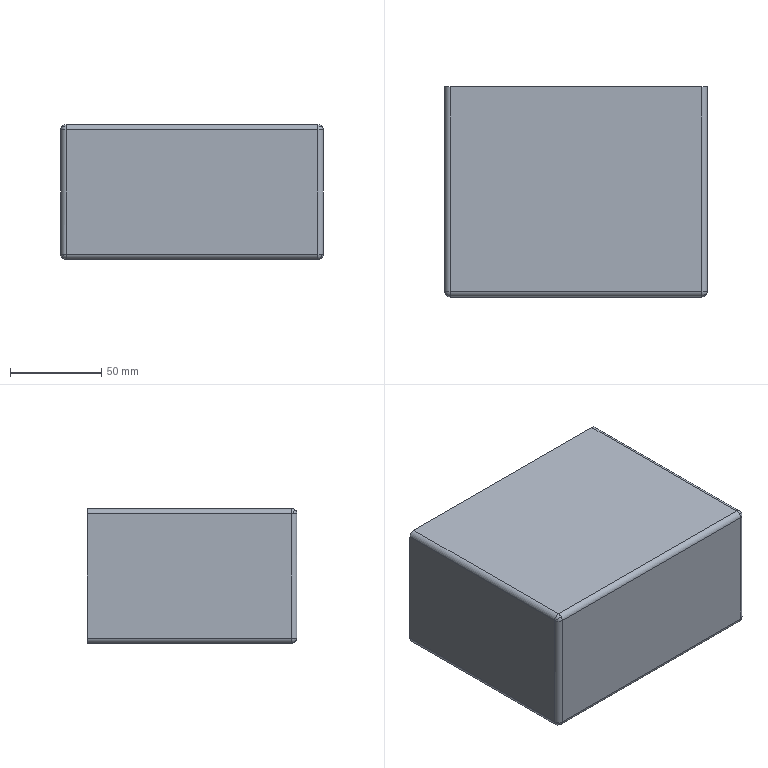Part | SolidWorks | features BaseBody 1 | 1 solid | 22 faces | box 144 x 115 x 74 mm | volume 1223728 mm3 | sphere 8 | cylinder 8 | plane 6 | commonest cylinder face diameters 6 x8
STEP:
#1=CARTESIAN_POINT('',(69.,-150.,-34.));
#2=VERTEX_POINT('',#1);
#3=CARTESIAN_POINT('',(69.,-147.,-37.));
#4=VERTEX_POINT('',#3);
#5=CARTESIAN_POINT('',(69.,-147.,-34.));
#6=DIRECTION('',(1.,0.,0.));
#7=DIRECTION('',(0.,-1.,0.));
#8=AXIS2_PLACEMENT_3D('',#5,#6,#7);
#9=CIRCLE('',#8,3.);
#10=EDGE_CURVE('',#2,#4,#9,.T.);
#11=ORIENTED_EDGE('',*,*,#10,.T.);
#12=CARTESIAN_POINT('',(71.121,-149.121,-34.));
#13=VERTEX_POINT('',#12);
#14=CARTESIAN_POINT('',(69.,-147.,-34.));
#15=DIRECTION('',(-0.7071,-0.7071,0.));
#16=DIRECTION('',(0.7071,-0.7071,0.));
#17=AXIS2_PLACEMENT_3D('',#14,#15,#16);
#18=CIRCLE('',#17,3.);
#19=EDGE_CURVE('',#4,#13,#18,.T.);
#20=ORIENTED_EDGE('',*,*,#19,.T.);
#21=CARTESIAN_POINT('',(69.,-147.,-34.));
#22=DIRECTION('',(0.,0.,-1.));
#23=DIRECTION('',(1.,0.,0.));
#24=AXIS2_PLACEMENT_3D('',#21,#22,#23);
#25=CIRCLE('',#24,3.);
#26=EDGE_CURVE('',#13,#2,#25,.T.);
#27=ORIENTED_EDGE('',*,*,#26,.T.);
#28=EDGE_LOOP('',(#11,#20,#27));
#29=FACE_OUTER_BOUND('',#28,.T.);
#30=CARTESIAN_POINT('',(69.,-147.,-34.));
#31=DIRECTION('',(-0.7071,-0.7071,0.));
#32=DIRECTION('',(-0.5774,0.5774,0.5774));
#33=AXIS2_PLACEMENT_3D('',#30,#31,#32);
#34=SPHERICAL_SURFACE('',#33,3.);
#35=ADVANCED_FACE('',(#29),#34,.T.);
#36=CARTESIAN_POINT('',(69.,-147.,37.));
#37=VERTEX_POINT('',#36);
#38=CARTESIAN_POINT('',(69.,-149.121,36.121));
#39=VERTEX_POINT('',#38);
#40=CARTESIAN_POINT('',(69.,-147.,34.));
#41=DIRECTION('',(1.,0.,0.));
#42=DIRECTION('',(0.,0.,1.));
#43=AXIS2_PLACEMENT_3D('',#40,#41,#42);
#44=CIRCLE('',#43,3.);
#45=EDGE_CURVE('',#37,#39,#44,.T.);
#46=ORIENTED_EDGE('',*,*,#45,.T.);
#47=CARTESIAN_POINT('',(72.,-147.,34.));
#48=VERTEX_POINT('',#47);
#49=CARTESIAN_POINT('',(69.,-147.,34.));
#50=DIRECTION('',(0.,0.7071,0.7071));
#51=DIRECTION('',(0.,-0.7071,0.7071));
#52=AXIS2_PLACEMENT_3D('',#49,#50,#51);
#53=CIRCLE('',#52,3.);
#54=EDGE_CURVE('',#39,#48,#53,.T.);
#55=ORIENTED_EDGE('',*,*,#54,.T.);
#56=CARTESIAN_POINT('',(69.,-147.,34.));
#57=DIRECTION('',(0.,-1.,0.));
#58=DIRECTION('',(1.,0.,0.));
#59=AXIS2_PLACEMENT_3D('',#56,#57,#58);
#60=CIRCLE('',#59,3.);
#61=EDGE_CURVE('',#48,#37,#60,.T.);
#62=ORIENTED_EDGE('',*,*,#61,.T.);
#63=EDGE_LOOP('',(#46,#55,#62));
#64=FACE_OUTER_BOUND('',#63,.T.);
#65=CARTESIAN_POINT('',(69.,-147.,34.));
#66=DIRECTION('',(0.,0.7071,0.7071));
#67=DIRECTION('',(-0.5774,0.5774,-0.5774));
#68=AXIS2_PLACEMENT_3D('',#65,#66,#67);
#69=SPHERICAL_SURFACE('',#68,3.);
#70=ADVANCED_FACE('',(#64),#69,.T.);
#71=CARTESIAN_POINT('',(-69.,-150.,-34.));
#72=VERTEX_POINT('',#71);
#73=CARTESIAN_POINT('',(-70.342,-149.683,-34.));
#74=VERTEX_POINT('',#73);
#75=CARTESIAN_POINT('',(-69.,-147.,-34.));
#76=DIRECTION('',(0.,0.,-1.));
#77=DIRECTION('',(0.,-1.,0.));
#78=AXIS2_PLACEMENT_3D('',#75,#76,#77);
#79=CIRCLE('',#78,3.);
#80=EDGE_CURVE('',#72,#74,#79,.T.);
#81=ORIENTED_EDGE('',*,*,#80,.T.);
#82=CARTESIAN_POINT('',(-70.342,-147.,-36.683));
#83=VERTEX_POINT('',#82);
#84=CARTESIAN_POINT('',(-69.,-147.,-34.));
#85=DIRECTION('',(0.8165,-0.4082,-0.4082));
#86=DIRECTION('',(0.4472,0.8944,0.));
#87=AXIS2_PLACEMENT_3D('',#84,#85,#86);
#88=CIRCLE('',#87,3.);
#89=EDGE_CURVE('',#74,#83,#88,.T.);
#90=ORIENTED_EDGE('',*,*,#89,.T.);
#91=CARTESIAN_POINT('',(-69.,-147.,-37.));
#92=VERTEX_POINT('',#91);
#93=CARTESIAN_POINT('',(-69.,-147.,-34.));
#94=DIRECTION('',(0.,-1.,0.));
#95=DIRECTION('',(-1.,0.,0.));
#96=AXIS2_PLACEMENT_3D('',#93,#94,#95);
#97=CIRCLE('',#96,3.);
#98=EDGE_CURVE('',#83,#92,#97,.T.);
#99=ORIENTED_EDGE('',*,*,#98,.T.);
#100=CARTESIAN_POINT('',(-69.,-147.,-34.));
#101=DIRECTION('',(-1.,0.,0.));
#102=DIRECTION('',(0.,0.,-1.));
#103=AXIS2_PLACEMENT_3D('',#100,#101,#102);
#104=CIRCLE('',#103,3.);
#105=EDGE_CURVE('',#92,#72,#104,.T.);
#106=ORIENTED_EDGE('',*,*,#105,.T.);
#107=EDGE_LOOP('',(#81,#90,#99,#106));
#108=FACE_OUTER_BOUND('',#107,.T.);
#109=CARTESIAN_POINT('',(-69.,-147.,-34.));
#110=DIRECTION('',(0.8165,-0.4082,-0.4082));
#111=DIRECTION('',(0.5774,0.5774,0.5774));
#112=AXIS2_PLACEMENT_3D('',#109,#110,#111);
#113=SPHERICAL_SURFACE('',#112,3.);
#114=ADVANCED_FACE('',(#108),#113,.T.);
#115=CARTESIAN_POINT('',(-69.,-147.,37.));
#116=VERTEX_POINT('',#115);
#117=CARTESIAN_POINT('',(-72.,-147.,34.));
#118=VERTEX_POINT('',#117);
#119=CARTESIAN_POINT('',(-69.,-147.,34.));
#120=DIRECTION('',(0.,-1.,0.));
#121=DIRECTION('',(0.,0.,1.));
#122=AXIS2_PLACEMENT_3D('',#119,#120,#121);
#123=CIRCLE('',#122,3.);
#124=EDGE_CURVE('',#116,#118,#123,.T.);
#125=ORIENTED_EDGE('',*,*,#124,.T.);
#126=CARTESIAN_POINT('',(-69.,-149.121,36.121));
#127=VERTEX_POINT('',#126);
#128=CARTESIAN_POINT('',(-69.,-147.,34.));
#129=DIRECTION('',(0.,0.7071,0.7071));
#130=DIRECTION('',(0.,-0.7071,0.7071));
#131=AXIS2_PLACEMENT_3D('',#128,#129,#130);
#132=CIRCLE('',#131,3.);
#133=EDGE_CURVE('',#118,#127,#132,.T.);
#134=ORIENTED_EDGE('',*,*,#133,.T.);
#135=CARTESIAN_POINT('',(-69.,-147.,34.));
#136=DIRECTION('',(-1.,0.,0.));
#137=DIRECTION('',(0.,-1.,0.));
#138=AXIS2_PLACEMENT_3D('',#135,#136,#137);
#139=CIRCLE('',#138,3.);
#140=EDGE_CURVE('',#127,#116,#139,.T.);
#141=ORIENTED_EDGE('',*,*,#140,.T.);
#142=EDGE_LOOP('',(#125,#134,#141));
#143=FACE_OUTER_BOUND('',#142,.T.);
#144=CARTESIAN_POINT('',(-69.,-147.,34.));
#145=DIRECTION('',(0.,0.7071,0.7071));
#146=DIRECTION('',(0.5774,0.5774,-0.5774));
#147=AXIS2_PLACEMENT_3D('',#144,#145,#146);
#148=SPHERICAL_SURFACE('',#147,3.);
#149=ADVANCED_FACE('',(#143),#148,.T.);
#150=CARTESIAN_POINT('',(-72.,-35.,34.));
#151=VERTEX_POINT('',#150);
#152=CARTESIAN_POINT('',(-72.,-35.,34.));
#153=DIRECTION('',(0.,-1.,0.));
#154=VECTOR('',#153,1000.);
#155=LINE('',#152,#154);
#156=EDGE_CURVE('',#151,#118,#155,.T.);
#157=ORIENTED_EDGE('',*,*,#156,.F.);
#158=CARTESIAN_POINT('',(-72.,-35.,-34.));
#159=VERTEX_POINT('',#158);
#160=CARTESIAN_POINT('',(-72.,-35.,-34.));
#161=DIRECTION('',(0.,0.,1.));
#162=VECTOR('',#161,1000.);
#163=LINE('',#160,#162);
#164=EDGE_CURVE('',#159,#151,#163,.T.);
#165=ORIENTED_EDGE('',*,*,#164,.F.);
#166=CARTESIAN_POINT('',(-72.,-147.,-34.));
#167=VERTEX_POINT('',#166);
#168=CARTESIAN_POINT('',(-72.,-147.,-34.));
#169=DIRECTION('',(0.,1.,0.));
#170=VECTOR('',#169,1000.);
#171=LINE('',#168,#170);
#172=EDGE_CURVE('',#167,#159,#171,.T.);
#173=ORIENTED_EDGE('',*,*,#172,.F.);
#174=CARTESIAN_POINT('',(-72.,-147.,34.));
#175=DIRECTION('',(0.,0.,-1.));
#176=VECTOR('',#175,1000.);
#177=LINE('',#174,#176);
#178=EDGE_CURVE('',#118,#167,#177,.T.);
#179=ORIENTED_EDGE('',*,*,#178,.F.);
#180=EDGE_LOOP('',(#157,#165,#173,#179));
#181=FACE_OUTER_BOUND('',#180,.T.);
#182=CARTESIAN_POINT('',(-72.,-150.,-37.));
#183=DIRECTION('',(-1.,0.,0.));
#184=DIRECTION('',(0.,0.,1.));
#185=AXIS2_PLACEMENT_3D('',#182,#183,#184);
#186=PLANE('',#185);
#187=ADVANCED_FACE('',(#181),#186,.T.);
#188=CARTESIAN_POINT('',(69.,-35.,37.));
#189=VERTEX_POINT('',#188);
#190=CARTESIAN_POINT('',(69.,-35.,37.));
#191=DIRECTION('',(0.,-1.,0.));
#192=VECTOR('',#191,1000.);
#193=LINE('',#190,#192);
#194=EDGE_CURVE('',#189,#37,#193,.T.);
#195=ORIENTED_EDGE('',*,*,#194,.F.);
#196=CARTESIAN_POINT('',(-69.,-35.,37.));
#197=VERTEX_POINT('',#196);
#198=CARTESIAN_POINT('',(-69.,-35.,37.));
#199=DIRECTION('',(1.,0.,0.));
#200=VECTOR('',#199,1000.);
#201=LINE('',#198,#200);
#202=EDGE_CURVE('',#197,#189,#201,.T.);
#203=ORIENTED_EDGE('',*,*,#202,.F.);
#204=CARTESIAN_POINT('',(-69.,-147.,37.));
#205=DIRECTION('',(0.,1.,0.));
#206=VECTOR('',#205,1000.);
#207=LINE('',#204,#206);
#208=EDGE_CURVE('',#116,#197,#207,.T.);
#209=ORIENTED_EDGE('',*,*,#208,.F.);
#210=CARTESIAN_POINT('',(69.,-147.,37.));
#211=DIRECTION('',(-1.,0.,0.));
#212=VECTOR('',#211,1000.);
#213=LINE('',#210,#212);
#214=EDGE_CURVE('',#37,#116,#213,.T.);
#215=ORIENTED_EDGE('',*,*,#214,.F.);
#216=EDGE_LOOP('',(#195,#203,#209,#215));
#217=FACE_OUTER_BOUND('',#216,.T.);
#218=CARTESIAN_POINT('',(-72.,-150.,37.));
#219=DIRECTION('',(0.,0.,1.));
#220=DIRECTION('',(1.,0.,0.));
#221=AXIS2_PLACEMENT_3D('',#218,#219,#220);
#222=PLANE('',#221);
#223=ADVANCED_FACE('',(#217),#222,.T.);
#224=CARTESIAN_POINT('',(-69.,-150.,34.));
#225=VERTEX_POINT('',#224);
#226=CARTESIAN_POINT('',(-69.,-150.,-34.));
#227=DIRECTION('',(0.,0.,1.));
#228=VECTOR('',#227,1000.);
#229=LINE('',#226,#228);
#230=EDGE_CURVE('',#72,#225,#229,.T.);
#231=ORIENTED_EDGE('',*,*,#230,.F.);
#232=CARTESIAN_POINT('',(69.,-150.,-34.));
#233=DIRECTION('',(-1.,0.,0.));
#234=VECTOR('',#233,1000.);
#235=LINE('',#232,#234);
#236=EDGE_CURVE('',#2,#72,#235,.T.);
#237=ORIENTED_EDGE('',*,*,#236,.F.);
#238=CARTESIAN_POINT('',(69.,-150.,34.));
#239=VERTEX_POINT('',#238);
#240=CARTESIAN_POINT('',(69.,-150.,34.));
#241=DIRECTION('',(0.,0.,-1.));
#242=VECTOR('',#241,1000.);
#243=LINE('',#240,#242);
#244=EDGE_CURVE('',#239,#2,#243,.T.);
#245=ORIENTED_EDGE('',*,*,#244,.F.);
#246=CARTESIAN_POINT('',(-69.,-150.,34.));
#247=DIRECTION('',(1.,0.,0.));
#248=VECTOR('',#247,1000.);
#249=LINE('',#246,#248);
#250=EDGE_CURVE('',#225,#239,#249,.T.);
#251=ORIENTED_EDGE('',*,*,#250,.F.);
#252=EDGE_LOOP('',(#231,#237,#245,#251));
#253=FACE_OUTER_BOUND('',#252,.T.);
#254=CARTESIAN_POINT('',(0.,-150.,0.));
#255=DIRECTION('',(0.,-1.,0.));
#256=DIRECTION('',(0.,0.,-1.));
#257=AXIS2_PLACEMENT_3D('',#254,#255,#256);
#258=PLANE('',#257);
#259=ADVANCED_FACE('',(#253),#258,.T.);
#260=CARTESIAN_POINT('',(72.,-35.,34.));
#261=VERTEX_POINT('',#260);
#262=CARTESIAN_POINT('',(69.,-35.,34.));
#263=DIRECTION('',(0.,-1.,0.));
#264=DIRECTION('',(1.,0.,0.));
#265=AXIS2_PLACEMENT_3D('',#262,#263,#264);
#266=CIRCLE('',#265,3.);
#267=EDGE_CURVE('',#261,#189,#266,.T.);
#268=ORIENTED_EDGE('',*,*,#267,.F.);
#269=CARTESIAN_POINT('',(72.,-35.,-34.));
#270=VERTEX_POINT('',#269);
#271=CARTESIAN_POINT('',(72.,-35.,-34.));
#272=DIRECTION('',(0.,0.,1.));
#273=VECTOR('',#272,1000.);
#274=LINE('',#271,#273);
#275=EDGE_CURVE('',#270,#261,#274,.T.);
#276=ORIENTED_EDGE('',*,*,#275,.F.);
#277=CARTESIAN_POINT('',(69.,-35.,-37.));
#278=VERTEX_POINT('',#277);
#279=CARTESIAN_POINT('',(69.,-35.,-34.));
#280=DIRECTION('',(0.,-1.,0.));
#281=DIRECTION('',(0.,0.,-1.));
#282=AXIS2_PLACEMENT_3D('',#279,#280,#281);
#283=CIRCLE('',#282,3.);
#284=EDGE_CURVE('',#278,#270,#283,.T.);
#285=ORIENTED_EDGE('',*,*,#284,.F.);
#286=CARTESIAN_POINT('',(-69.,-35.,-37.));
#287=VERTEX_POINT('',#286);
#288=CARTESIAN_POINT('',(-69.,-35.,-37.));
#289=DIRECTION('',(1.,0.,0.));
#290=VECTOR('',#289,1000.);
#291=LINE('',#288,#290);
#292=EDGE_CURVE('',#287,#278,#291,.T.);
#293=ORIENTED_EDGE('',*,*,#292,.F.);
#294=CARTESIAN_POINT('',(-69.,-35.,-34.));
#295=DIRECTION('',(0.,-1.,0.));
#296=DIRECTION('',(-1.,0.,0.));
#297=AXIS2_PLACEMENT_3D('',#294,#295,#296);
#298=CIRCLE('',#297,3.);
#299=EDGE_CURVE('',#159,#287,#298,.T.);
#300=ORIENTED_EDGE('',*,*,#299,.F.);
#301=ORIENTED_EDGE('',*,*,#164,.T.);
#302=CARTESIAN_POINT('',(-69.,-35.,34.));
#303=DIRECTION('',(0.,-1.,0.));
#304=DIRECTION('',(0.,0.,1.));
#305=AXIS2_PLACEMENT_3D('',#302,#303,#304);
#306=CIRCLE('',#305,3.);
#307=EDGE_CURVE('',#197,#151,#306,.T.);
#308=ORIENTED_EDGE('',*,*,#307,.F.);
#309=ORIENTED_EDGE('',*,*,#202,.T.);
#310=EDGE_LOOP('',(#268,#276,#285,#293,#300,#301,#308,#309));
#311=FACE_OUTER_BOUND('',#310,.T.);
#312=CARTESIAN_POINT('',(0.,-35.,0.));
#313=DIRECTION('',(0.,1.,0.));
#314=DIRECTION('',(1.,0.,0.));
#315=AXIS2_PLACEMENT_3D('',#312,#313,#314);
#316=PLANE('',#315);
#317=ADVANCED_FACE('',(#311),#316,.T.);
#318=CARTESIAN_POINT('',(69.,-147.,-37.));
#319=DIRECTION('',(0.,1.,0.));
#320=VECTOR('',#319,1000.);
#321=LINE('',#318,#320);
#322=EDGE_CURVE('',#4,#278,#321,.T.);
#323=ORIENTED_EDGE('',*,*,#322,.F.);
#324=CARTESIAN_POINT('',(-69.,-147.,-37.));
#325=DIRECTION('',(1.,0.,0.));
#326=VECTOR('',#325,1000.);
#327=LINE('',#324,#326);
#328=EDGE_CURVE('',#92,#4,#327,.T.);
#329=ORIENTED_EDGE('',*,*,#328,.F.);
#330=CARTESIAN_POINT('',(-69.,-35.,-37.));
#331=DIRECTION('',(0.,-1.,0.));
#332=VECTOR('',#331,1000.);
#333=LINE('',#330,#332);
#334=EDGE_CURVE('',#287,#92,#333,.T.);
#335=ORIENTED_EDGE('',*,*,#334,.F.);
#336=ORIENTED_EDGE('',*,*,#292,.T.);
#337=EDGE_LOOP('',(#323,#329,#335,#336));
#338=FACE_OUTER_BOUND('',#337,.T.);
#339=CARTESIAN_POINT('',(72.,-150.,-37.));
#340=DIRECTION('',(0.,0.,-1.));
#341=DIRECTION('',(0.,-1.,0.));
#342=AXIS2_PLACEMENT_3D('',#339,#340,#341);
#343=PLANE('',#342);
#344=ADVANCED_FACE('',(#338),#343,.T.);
#345=CARTESIAN_POINT('',(72.,-147.,34.));
#346=DIRECTION('',(0.,1.,0.));
#347=VECTOR('',#346,1000.);
#348=LINE('',#345,#347);
#349=EDGE_CURVE('',#48,#261,#348,.T.);
#350=ORIENTED_EDGE('',*,*,#349,.F.);
#351=CARTESIAN_POINT('',(72.,-147.,-34.));
#352=VERTEX_POINT('',#351);
#353=CARTESIAN_POINT('',(72.,-147.,-34.));
#354=DIRECTION('',(0.,0.,1.));
#355=VECTOR('',#354,1000.);
#356=LINE('',#353,#355);
#357=EDGE_CURVE('',#352,#48,#356,.T.);
#358=ORIENTED_EDGE('',*,*,#357,.F.);
#359=CARTESIAN_POINT('',(72.,-35.,-34.));
#360=DIRECTION('',(0.,-1.,0.));
#361=VECTOR('',#360,1000.);
#362=LINE('',#359,#361);
#363=EDGE_CURVE('',#270,#352,#362,.T.);
#364=ORIENTED_EDGE('',*,*,#363,.F.);
#365=ORIENTED_EDGE('',*,*,#275,.T.);
#366=EDGE_LOOP('',(#350,#358,#364,#365));
#367=FACE_OUTER_BOUND('',#366,.T.);
#368=CARTESIAN_POINT('',(72.,-150.,37.));
#369=DIRECTION('',(1.,0.,0.));
#370=DIRECTION('',(0.,0.,1.));
#371=AXIS2_PLACEMENT_3D('',#368,#369,#370);
#372=PLANE('',#371);
#373=ADVANCED_FACE('',(#367),#372,.T.);
#374=ORIENTED_EDGE('',*,*,#284,.T.);
#375=ORIENTED_EDGE('',*,*,#363,.T.);
#376=CARTESIAN_POINT('',(69.,-147.,-34.));
#377=DIRECTION('',(0.,-1.,0.));
#378=DIRECTION('',(0.,0.,-1.));
#379=AXIS2_PLACEMENT_3D('',#376,#377,#378);
#380=CIRCLE('',#379,3.);
#381=EDGE_CURVE('',#4,#352,#380,.T.);
#382=ORIENTED_EDGE('',*,*,#381,.F.);
#383=ORIENTED_EDGE('',*,*,#322,.T.);
#384=EDGE_LOOP('',(#374,#375,#382,#383));
#385=FACE_OUTER_BOUND('',#384,.T.);
#386=CARTESIAN_POINT('',(69.,-147.,-34.));
#387=DIRECTION('',(0.,1.,0.));
#388=DIRECTION('',(0.,0.,-1.));
#389=AXIS2_PLACEMENT_3D('',#386,#387,#388);
#390=CYLINDRICAL_SURFACE('',#389,3.);
#391=ADVANCED_FACE('',(#385),#390,.T.);
#392=ORIENTED_EDGE('',*,*,#105,.F.);
#393=ORIENTED_EDGE('',*,*,#328,.T.);
#394=ORIENTED_EDGE('',*,*,#10,.F.);
#395=ORIENTED_EDGE('',*,*,#236,.T.);
#396=EDGE_LOOP('',(#392,#393,#394,#395));
#397=FACE_OUTER_BOUND('',#396,.T.);
#398=CARTESIAN_POINT('',(69.,-147.,-34.));
#399=DIRECTION('',(-1.,0.,0.));
#400=DIRECTION('',(0.,-1.,0.));
#401=AXIS2_PLACEMENT_3D('',#398,#399,#400);
#402=CYLINDRICAL_SURFACE('',#401,3.);
#403=ADVANCED_FACE('',(#397),#402,.T.);
#404=ORIENTED_EDGE('',*,*,#299,.T.);
#405=ORIENTED_EDGE('',*,*,#334,.T.);
#406=ORIENTED_EDGE('',*,*,#98,.F.);
#407=CARTESIAN_POINT('',(-69.,-147.,-34.));
#408=DIRECTION('',(0.,-1.,0.));
#409=DIRECTION('',(-1.,0.,0.));
#410=AXIS2_PLACEMENT_3D('',#407,#408,#409);
#411=CIRCLE('',#410,3.);
#412=EDGE_CURVE('',#167,#83,#411,.T.);
#413=ORIENTED_EDGE('',*,*,#412,.F.);
#414=ORIENTED_EDGE('',*,*,#172,.T.);
#415=EDGE_LOOP('',(#404,#405,#406,#413,#414));
#416=FACE_OUTER_BOUND('',#415,.T.);
#417=CARTESIAN_POINT('',(-69.,-147.,-34.));
#418=DIRECTION('',(0.,1.,0.));
#419=DIRECTION('',(-1.,0.,0.));
#420=AXIS2_PLACEMENT_3D('',#417,#418,#419);
#421=CYLINDRICAL_SURFACE('',#420,3.);
#422=ADVANCED_FACE('',(#416),#421,.T.);
#423=ORIENTED_EDGE('',*,*,#307,.T.);
#424=ORIENTED_EDGE('',*,*,#156,.T.);
#425=ORIENTED_EDGE('',*,*,#124,.F.);
#426=ORIENTED_EDGE('',*,*,#208,.T.);
#427=EDGE_LOOP('',(#423,#424,#425,#426));
#428=FACE_OUTER_BOUND('',#427,.T.);
#429=CARTESIAN_POINT('',(-69.,-147.,34.));
#430=DIRECTION('',(0.,1.,0.));
#431=DIRECTION('',(0.,0.,1.));
#432=AXIS2_PLACEMENT_3D('',#429,#430,#431);
#433=CYLINDRICAL_SURFACE('',#432,3.);
#434=ADVANCED_FACE('',(#428),#433,.T.);
#435=ORIENTED_EDGE('',*,*,#45,.F.);
#436=ORIENTED_EDGE('',*,*,#214,.T.);
#437=ORIENTED_EDGE('',*,*,#140,.F.);
#438=CARTESIAN_POINT('',(-69.,-147.,34.));
#439=DIRECTION('',(-1.,0.,0.));
#440=DIRECTION('',(0.,-1.,0.));
#441=AXIS2_PLACEMENT_3D('',#438,#439,#440);
#442=CIRCLE('',#441,3.);
#443=EDGE_CURVE('',#225,#127,#442,.T.);
#444=ORIENTED_EDGE('',*,*,#443,.F.);
#445=ORIENTED_EDGE('',*,*,#250,.T.);
#446=CARTESIAN_POINT('',(69.,-147.,34.));
#447=DIRECTION('',(1.,0.,0.));
#448=DIRECTION('',(0.,0.,1.));
#449=AXIS2_PLACEMENT_3D('',#446,#447,#448);
#450=CIRCLE('',#449,3.);
#451=EDGE_CURVE('',#39,#239,#450,.T.);
#452=ORIENTED_EDGE('',*,*,#451,.F.);
#453=EDGE_LOOP('',(#435,#436,#437,#444,#445,#452));
#454=FACE_OUTER_BOUND('',#453,.T.);
#455=CARTESIAN_POINT('',(-69.,-147.,34.));
#456=DIRECTION('',(1.,0.,0.));
#457=DIRECTION('',(0.,-1.,0.));
#458=AXIS2_PLACEMENT_3D('',#455,#456,#457);
#459=CYLINDRICAL_SURFACE('',#458,3.);
#460=ADVANCED_FACE('',(#454),#459,.T.);
#461=CARTESIAN_POINT('',(-69.,-147.,34.));
#462=DIRECTION('',(0.,0.,1.));
#463=DIRECTION('',(-1.,0.,0.));
#464=AXIS2_PLACEMENT_3D('',#461,#462,#463);
#465=CIRCLE('',#464,3.);
#466=EDGE_CURVE('',#118,#225,#465,.T.);
#467=ORIENTED_EDGE('',*,*,#466,.F.);
#468=ORIENTED_EDGE('',*,*,#178,.T.);
#469=CARTESIAN_POINT('',(-69.,-147.,-34.));
#470=DIRECTION('',(0.,0.,-1.));
#471=DIRECTION('',(0.,-1.,0.));
#472=AXIS2_PLACEMENT_3D('',#469,#470,#471);
#473=CIRCLE('',#472,3.);
#474=EDGE_CURVE('',#74,#167,#473,.T.);
#475=ORIENTED_EDGE('',*,*,#474,.F.);
#476=ORIENTED_EDGE('',*,*,#80,.F.);
#477=ORIENTED_EDGE('',*,*,#230,.T.);
#478=EDGE_LOOP('',(#467,#468,#475,#476,#477));
#479=FACE_OUTER_BOUND('',#478,.T.);
#480=CARTESIAN_POINT('',(-69.,-147.,-34.));
#481=DIRECTION('',(0.,0.,1.));
#482=DIRECTION('',(0.,-1.,0.));
#483=AXIS2_PLACEMENT_3D('',#480,#481,#482);
#484=CYLINDRICAL_SURFACE('',#483,3.);
#485=ADVANCED_FACE('',(#479),#484,.T.);
#486=ORIENTED_EDGE('',*,*,#133,.F.);
#487=ORIENTED_EDGE('',*,*,#466,.T.);
#488=ORIENTED_EDGE('',*,*,#443,.T.);
#489=EDGE_LOOP('',(#486,#487,#488));
#490=FACE_OUTER_BOUND('',#489,.T.);
#491=CARTESIAN_POINT('',(-69.,-147.,34.));
#492=DIRECTION('',(0.,0.7071,0.7071));
#493=DIRECTION('',(0.5774,0.5774,-0.5774));
#494=AXIS2_PLACEMENT_3D('',#491,#492,#493);
#495=SPHERICAL_SURFACE('',#494,3.);
#496=ADVANCED_FACE('',(#490),#495,.T.);
#497=ORIENTED_EDGE('',*,*,#89,.F.);
#498=ORIENTED_EDGE('',*,*,#474,.T.);
#499=ORIENTED_EDGE('',*,*,#412,.T.);
#500=EDGE_LOOP('',(#497,#498,#499));
#501=FACE_OUTER_BOUND('',#500,.T.);
#502=CARTESIAN_POINT('',(-69.,-147.,-34.));
#503=DIRECTION('',(0.8165,-0.4082,-0.4082));
#504=DIRECTION('',(0.5774,0.5774,0.5774));
#505=AXIS2_PLACEMENT_3D('',#502,#503,#504);
#506=SPHERICAL_SURFACE('',#505,3.);
#507=ADVANCED_FACE('',(#501),#506,.T.);
#508=ORIENTED_EDGE('',*,*,#267,.T.);
#509=ORIENTED_EDGE('',*,*,#194,.T.);
#510=ORIENTED_EDGE('',*,*,#61,.F.);
#511=ORIENTED_EDGE('',*,*,#349,.T.);
#512=EDGE_LOOP('',(#508,#509,#510,#511));
#513=FACE_OUTER_BOUND('',#512,.T.);
#514=CARTESIAN_POINT('',(69.,-147.,34.));
#515=DIRECTION('',(0.,1.,0.));
#516=DIRECTION('',(1.,0.,0.));
#517=AXIS2_PLACEMENT_3D('',#514,#515,#516);
#518=CYLINDRICAL_SURFACE('',#517,3.);
#519=ADVANCED_FACE('',(#513),#518,.T.);
#520=CARTESIAN_POINT('',(69.,-147.,-34.));
#521=DIRECTION('',(0.,0.,-1.));
#522=DIRECTION('',(1.,0.,0.));
#523=AXIS2_PLACEMENT_3D('',#520,#521,#522);
#524=CIRCLE('',#523,3.);
#525=EDGE_CURVE('',#352,#13,#524,.T.);
#526=ORIENTED_EDGE('',*,*,#525,.F.);
#527=ORIENTED_EDGE('',*,*,#357,.T.);
#528=CARTESIAN_POINT('',(69.,-147.,34.));
#529=DIRECTION('',(0.,0.,1.));
#530=DIRECTION('',(0.,-1.,0.));
#531=AXIS2_PLACEMENT_3D('',#528,#529,#530);
#532=CIRCLE('',#531,3.);
#533=EDGE_CURVE('',#239,#48,#532,.T.);
#534=ORIENTED_EDGE('',*,*,#533,.F.);
#535=ORIENTED_EDGE('',*,*,#244,.T.);
#536=ORIENTED_EDGE('',*,*,#26,.F.);
#537=EDGE_LOOP('',(#526,#527,#534,#535,#536));
#538=FACE_OUTER_BOUND('',#537,.T.);
#539=CARTESIAN_POINT('',(69.,-147.,34.));
#540=DIRECTION('',(0.,0.,-1.));
#541=DIRECTION('',(0.,-1.,0.));
#542=AXIS2_PLACEMENT_3D('',#539,#540,#541);
#543=CYLINDRICAL_SURFACE('',#542,3.);
#544=ADVANCED_FACE('',(#538),#543,.T.);
#545=ORIENTED_EDGE('',*,*,#54,.F.);
#546=ORIENTED_EDGE('',*,*,#451,.T.);
#547=ORIENTED_EDGE('',*,*,#533,.T.);
#548=EDGE_LOOP('',(#545,#546,#547));
#549=FACE_OUTER_BOUND('',#548,.T.);
#550=CARTESIAN_POINT('',(69.,-147.,34.));
#551=DIRECTION('',(0.,0.7071,0.7071));
#552=DIRECTION('',(-0.5774,0.5774,-0.5774));
#553=AXIS2_PLACEMENT_3D('',#550,#551,#552);
#554=SPHERICAL_SURFACE('',#553,3.);
#555=ADVANCED_FACE('',(#549),#554,.T.);
#556=ORIENTED_EDGE('',*,*,#19,.F.);
#557=ORIENTED_EDGE('',*,*,#381,.T.);
#558=ORIENTED_EDGE('',*,*,#525,.T.);
#559=EDGE_LOOP('',(#556,#557,#558));
#560=FACE_OUTER_BOUND('',#559,.T.);
#561=CARTESIAN_POINT('',(69.,-147.,-34.));
#562=DIRECTION('',(-0.7071,-0.7071,0.));
#563=DIRECTION('',(-0.5774,0.5774,0.5774));
#564=AXIS2_PLACEMENT_3D('',#561,#562,#563);
#565=SPHERICAL_SURFACE('',#564,3.);
#566=ADVANCED_FACE('',(#560),#565,.T.);
#567=CLOSED_SHELL('',(#35,#70,#114,#149,#187,#223,#259,#317,#344,#373,#391,#403,#422,#434,#460,#485,#496,#507,#519,#544,#555,#566));
#568=MANIFOLD_SOLID_BREP('',#567);
#569=CARTESIAN_POINT('',(0.,0.,0.));
#570=DIRECTION('',(0.,0.,1.));
#571=DIRECTION('',(1.,0.,0.));
#572=AXIS2_PLACEMENT_3D('',#569,#570,#571);
#573=(LENGTH_UNIT()NAMED_UNIT(*)SI_UNIT(.MILLI.,.METRE.));
#574=UNCERTAINTY_MEASURE_WITH_UNIT(LENGTH_MEASURE(0.00001),#573,'','');
#575=(NAMED_UNIT(*)PLANE_ANGLE_UNIT()SI_UNIT($,.RADIAN.));
#576=(NAMED_UNIT(*)SI_UNIT($,.STERADIAN.)SOLID_ANGLE_UNIT());
#577=(GEOMETRIC_REPRESENTATION_CONTEXT(3)GLOBAL_UNCERTAINTY_ASSIGNED_CONTEXT((#574))GLOBAL_UNIT_ASSIGNED_CONTEXT((#573,#575,#576))REPRESENTATION_CONTEXT('',''));
#578=ADVANCED_BREP_SHAPE_REPRESENTATION('',(#568,#572),#577);